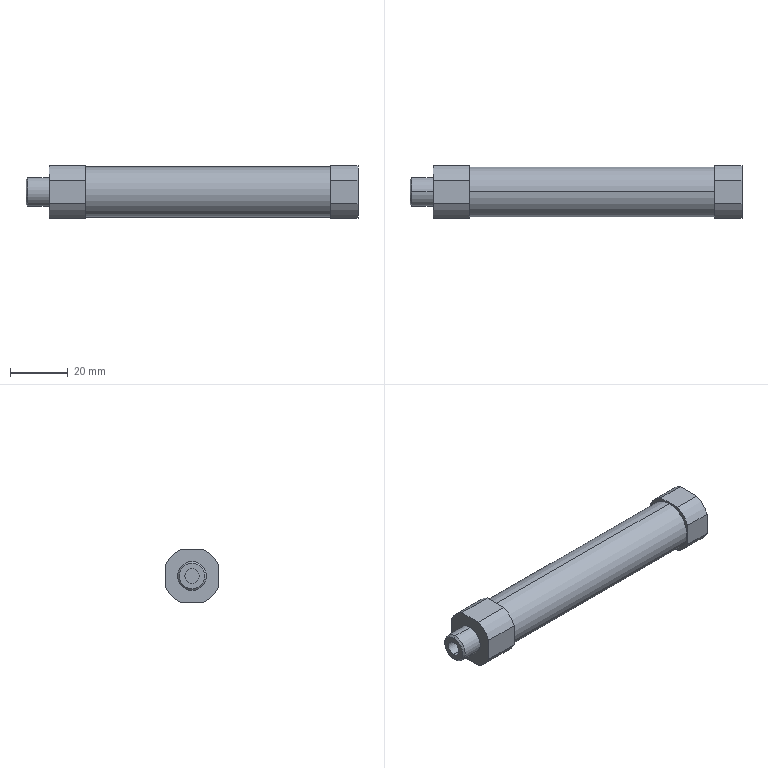Part | SolidWorks | features RefAxis 6, ICE 3, RevCut 3, 3DProfileFeature 2, Revolution 1 | 1 solid | 45 faces | box 115 x 18.3 x 18.3 mm | volume 13708 mm3 | cylinder 20 | plane 15 | cone 10 | commonest cylinder face diameters 20 x8 4.134 x4 5 x2 10 x2 16 x2 17.4 x2
STEP:
#1=CARTESIAN_POINT('',(77.5,0.,-8.));
#2=VERTEX_POINT('',#1);
#3=CARTESIAN_POINT('',(77.5,0.,8.));
#4=VERTEX_POINT('',#3);
#5=CARTESIAN_POINT('',(77.5,0.,0.));
#6=DIRECTION('',(-1.,0.,0.));
#7=DIRECTION('',(0.,0.,1.));
#8=AXIS2_PLACEMENT_3D('',#5,#6,#7);
#9=CIRCLE('',#8,8.);
#10=EDGE_CURVE('',#2,#4,#9,.T.);
#11=ORIENTED_EDGE('',*,*,#10,.F.);
#12=CARTESIAN_POINT('',(12.5,0.,-8.));
#13=VERTEX_POINT('',#12);
#14=CARTESIAN_POINT('',(50.,0.,-8.));
#15=DIRECTION('',(-1.,0.,0.));
#16=VECTOR('',#15,1000.);
#17=LINE('',#14,#16);
#18=EDGE_CURVE('',#2,#13,#17,.T.);
#19=ORIENTED_EDGE('',*,*,#18,.T.);
#20=CARTESIAN_POINT('',(12.5,0.,8.));
#21=VERTEX_POINT('',#20);
#22=CARTESIAN_POINT('',(12.5,0.,0.));
#23=DIRECTION('',(-1.,0.,0.));
#24=DIRECTION('',(0.,0.,1.));
#25=AXIS2_PLACEMENT_3D('',#22,#23,#24);
#26=CIRCLE('',#25,8.);
#27=EDGE_CURVE('',#13,#21,#26,.T.);
#28=ORIENTED_EDGE('',*,*,#27,.T.);
#29=CARTESIAN_POINT('',(50.,0.,8.));
#30=DIRECTION('',(-1.,0.,0.));
#31=VECTOR('',#30,1000.);
#32=LINE('',#29,#31);
#33=EDGE_CURVE('',#4,#21,#32,.T.);
#34=ORIENTED_EDGE('',*,*,#33,.F.);
#35=EDGE_LOOP('',(#11,#19,#28,#34));
#36=FACE_OUTER_BOUND('',#35,.T.);
#37=CARTESIAN_POINT('',(50.,0.,0.));
#38=DIRECTION('',(-1.,0.,0.));
#39=DIRECTION('',(0.,0.,1.));
#40=AXIS2_PLACEMENT_3D('',#37,#38,#39);
#41=CYLINDRICAL_SURFACE('',#40,8.);
#42=ADVANCED_FACE('',(#36),#41,.F.);
#43=CARTESIAN_POINT('',(12.5,0.,-2.5));
#44=VERTEX_POINT('',#43);
#45=CARTESIAN_POINT('',(12.5,0.,2.5));
#46=VERTEX_POINT('',#45);
#47=CARTESIAN_POINT('',(12.5,0.,0.));
#48=DIRECTION('',(-1.,0.,0.));
#49=DIRECTION('',(0.,0.,1.));
#50=AXIS2_PLACEMENT_3D('',#47,#48,#49);
#51=CIRCLE('',#50,2.5);
#52=EDGE_CURVE('',#44,#46,#51,.T.);
#53=ORIENTED_EDGE('',*,*,#52,.F.);
#54=CARTESIAN_POINT('',(-8.,0.,-2.5));
#55=VERTEX_POINT('',#54);
#56=CARTESIAN_POINT('',(50.,0.,-2.5));
#57=DIRECTION('',(-1.,0.,0.));
#58=VECTOR('',#57,1000.);
#59=LINE('',#56,#58);
#60=EDGE_CURVE('',#44,#55,#59,.T.);
#61=ORIENTED_EDGE('',*,*,#60,.T.);
#62=CARTESIAN_POINT('',(-8.,0.,2.5));
#63=VERTEX_POINT('',#62);
#64=CARTESIAN_POINT('',(-8.,0.,0.));
#65=DIRECTION('',(-1.,0.,0.));
#66=DIRECTION('',(0.,0.,1.));
#67=AXIS2_PLACEMENT_3D('',#64,#65,#66);
#68=CIRCLE('',#67,2.5);
#69=EDGE_CURVE('',#55,#63,#68,.T.);
#70=ORIENTED_EDGE('',*,*,#69,.T.);
#71=CARTESIAN_POINT('',(50.,0.,2.5));
#72=DIRECTION('',(-1.,0.,0.));
#73=VECTOR('',#72,1000.);
#74=LINE('',#71,#73);
#75=EDGE_CURVE('',#46,#63,#74,.T.);
#76=ORIENTED_EDGE('',*,*,#75,.F.);
#77=EDGE_LOOP('',(#53,#61,#70,#76));
#78=FACE_OUTER_BOUND('',#77,.T.);
#79=CARTESIAN_POINT('',(50.,0.,0.));
#80=DIRECTION('',(-1.,0.,0.));
#81=DIRECTION('',(0.,0.,1.));
#82=AXIS2_PLACEMENT_3D('',#79,#80,#81);
#83=CYLINDRICAL_SURFACE('',#82,2.5);
#84=ADVANCED_FACE('',(#78),#83,.F.);
#85=CARTESIAN_POINT('',(102.,2.457,0.));
#86=VERTEX_POINT('',#85);
#87=CARTESIAN_POINT('',(102.,3.65,2.067));
#88=VERTEX_POINT('',#87);
#89=CARTESIAN_POINT('',(102.,3.65,2.067));
#90=DIRECTION('',(0.,0.5,0.866));
#91=VECTOR('',#90,1000.);
#92=LINE('',#89,#91);
#93=EDGE_CURVE('',#86,#88,#92,.T.);
#94=ORIENTED_EDGE('',*,*,#93,.F.);
#95=CARTESIAN_POINT('',(102.,3.65,-2.067));
#96=VERTEX_POINT('',#95);
#97=CARTESIAN_POINT('',(102.,3.65,-2.067));
#98=DIRECTION('',(0.,0.5,-0.866));
#99=VECTOR('',#98,1000.);
#100=LINE('',#97,#99);
#101=EDGE_CURVE('',#86,#96,#100,.T.);
#102=ORIENTED_EDGE('',*,*,#101,.T.);
#103=CARTESIAN_POINT('',(102.,3.65,0.));
#104=DIRECTION('',(0.,-1.,0.));
#105=DIRECTION('',(0.,0.,-1.));
#106=AXIS2_PLACEMENT_3D('',#103,#104,#105);
#107=CIRCLE('',#106,2.067);
#108=EDGE_CURVE('',#88,#96,#107,.T.);
#109=ORIENTED_EDGE('',*,*,#108,.F.);
#110=EDGE_LOOP('',(#94,#102,#109));
#111=FACE_OUTER_BOUND('',#110,.T.);
#112=CARTESIAN_POINT('',(102.,3.65,0.));
#113=DIRECTION('',(0.,1.,0.));
#114=DIRECTION('',(0.,0.,1.));
#115=AXIS2_PLACEMENT_3D('',#112,#113,#114);
#116=CONICAL_SURFACE('',#115,2.067,1.047);
#117=ADVANCED_FACE('',(#111),#116,.F.);
#118=CARTESIAN_POINT('',(102.,8.717,2.067));
#119=VERTEX_POINT('',#118);
#120=CARTESIAN_POINT('',(102.,8.717,-2.067));
#121=VERTEX_POINT('',#120);
#122=CARTESIAN_POINT('',(102.,8.717,0.));
#123=DIRECTION('',(0.,-1.,0.));
#124=DIRECTION('',(0.,0.,-1.));
#125=AXIS2_PLACEMENT_3D('',#122,#123,#124);
#126=CIRCLE('',#125,2.067);
#127=EDGE_CURVE('',#119,#121,#126,.T.);
#128=ORIENTED_EDGE('',*,*,#127,.F.);
#129=CARTESIAN_POINT('',(102.,9.15,2.067));
#130=DIRECTION('',(0.,-1.,0.));
#131=VECTOR('',#130,1000.);
#132=LINE('',#129,#131);
#133=EDGE_CURVE('',#119,#88,#132,.T.);
#134=ORIENTED_EDGE('',*,*,#133,.T.);
#135=ORIENTED_EDGE('',*,*,#108,.T.);
#136=CARTESIAN_POINT('',(102.,9.15,-2.067));
#137=DIRECTION('',(0.,-1.,0.));
#138=VECTOR('',#137,1000.);
#139=LINE('',#136,#138);
#140=EDGE_CURVE('',#121,#96,#139,.T.);
#141=ORIENTED_EDGE('',*,*,#140,.F.);
#142=EDGE_LOOP('',(#128,#134,#135,#141));
#143=FACE_OUTER_BOUND('',#142,.T.);
#144=CARTESIAN_POINT('',(102.,9.15,0.));
#145=DIRECTION('',(0.,-1.,0.));
#146=DIRECTION('',(0.,0.,-1.));
#147=AXIS2_PLACEMENT_3D('',#144,#145,#146);
#148=CYLINDRICAL_SURFACE('',#147,2.067);
#149=ADVANCED_FACE('',(#143),#148,.F.);
#150=ORIENTED_EDGE('',*,*,#127,.T.);
#151=CARTESIAN_POINT('',(102.,9.15,-2.5));
#152=VERTEX_POINT('',#151);
#153=CARTESIAN_POINT('',(102.,9.15,-2.5));
#154=DIRECTION('',(0.,0.7071,-0.7071));
#155=VECTOR('',#154,1000.);
#156=LINE('',#153,#155);
#157=EDGE_CURVE('',#121,#152,#156,.T.);
#158=ORIENTED_EDGE('',*,*,#157,.T.);
#159=CARTESIAN_POINT('',(102.,9.15,2.5));
#160=VERTEX_POINT('',#159);
#161=CARTESIAN_POINT('',(102.,9.15,0.));
#162=DIRECTION('',(0.,-1.,0.));
#163=DIRECTION('',(0.,0.,-1.));
#164=AXIS2_PLACEMENT_3D('',#161,#162,#163);
#165=CIRCLE('',#164,2.5);
#166=EDGE_CURVE('',#160,#152,#165,.T.);
#167=ORIENTED_EDGE('',*,*,#166,.F.);
#168=CARTESIAN_POINT('',(102.,9.15,2.5));
#169=DIRECTION('',(0.,0.7071,0.7071));
#170=VECTOR('',#169,1000.);
#171=LINE('',#168,#170);
#172=EDGE_CURVE('',#119,#160,#171,.T.);
#173=ORIENTED_EDGE('',*,*,#172,.F.);
#174=EDGE_LOOP('',(#150,#158,#167,#173));
#175=FACE_OUTER_BOUND('',#174,.T.);
#176=CARTESIAN_POINT('',(102.,9.15,0.));
#177=DIRECTION('',(0.,1.,0.));
#178=DIRECTION('',(0.,0.,1.));
#179=AXIS2_PLACEMENT_3D('',#176,#177,#178);
#180=CONICAL_SURFACE('',#179,2.5,0.7854);
#181=ADVANCED_FACE('',(#175),#180,.F.);
#182=CARTESIAN_POINT('',(8.,8.717,2.067));
#183=VERTEX_POINT('',#182);
#184=CARTESIAN_POINT('',(8.,8.717,-2.067));
#185=VERTEX_POINT('',#184);
#186=CARTESIAN_POINT('',(8.,8.717,0.));
#187=DIRECTION('',(0.,-1.,0.));
#188=DIRECTION('',(0.,0.,-1.));
#189=AXIS2_PLACEMENT_3D('',#186,#187,#188);
#190=CIRCLE('',#189,2.067);
#191=EDGE_CURVE('',#183,#185,#190,.T.);
#192=ORIENTED_EDGE('',*,*,#191,.F.);
#193=CARTESIAN_POINT('',(8.,3.65,2.067));
#194=VERTEX_POINT('',#193);
#195=CARTESIAN_POINT('',(8.,9.15,2.067));
#196=DIRECTION('',(0.,-1.,0.));
#197=VECTOR('',#196,1000.);
#198=LINE('',#195,#197);
#199=EDGE_CURVE('',#183,#194,#198,.T.);
#200=ORIENTED_EDGE('',*,*,#199,.T.);
#201=CARTESIAN_POINT('',(8.,3.65,-2.067));
#202=VERTEX_POINT('',#201);
#203=CARTESIAN_POINT('',(8.,3.65,0.));
#204=DIRECTION('',(0.,-1.,0.));
#205=DIRECTION('',(0.,0.,-1.));
#206=AXIS2_PLACEMENT_3D('',#203,#204,#205);
#207=CIRCLE('',#206,2.067);
#208=EDGE_CURVE('',#194,#202,#207,.T.);
#209=ORIENTED_EDGE('',*,*,#208,.T.);
#210=CARTESIAN_POINT('',(8.,9.15,-2.067));
#211=DIRECTION('',(0.,-1.,0.));
#212=VECTOR('',#211,1000.);
#213=LINE('',#210,#212);
#214=EDGE_CURVE('',#185,#202,#213,.T.);
#215=ORIENTED_EDGE('',*,*,#214,.F.);
#216=EDGE_LOOP('',(#192,#200,#209,#215));
#217=FACE_OUTER_BOUND('',#216,.T.);
#218=CARTESIAN_POINT('',(8.,9.15,0.));
#219=DIRECTION('',(0.,-1.,0.));
#220=DIRECTION('',(0.,0.,-1.));
#221=AXIS2_PLACEMENT_3D('',#218,#219,#220);
#222=CYLINDRICAL_SURFACE('',#221,2.067);
#223=ADVANCED_FACE('',(#217),#222,.F.);
#224=ORIENTED_EDGE('',*,*,#191,.T.);
#225=CARTESIAN_POINT('',(8.,9.15,-2.5));
#226=VERTEX_POINT('',#225);
#227=CARTESIAN_POINT('',(8.,9.15,-2.5));
#228=DIRECTION('',(0.,0.7071,-0.7071));
#229=VECTOR('',#228,1000.);
#230=LINE('',#227,#229);
#231=EDGE_CURVE('',#185,#226,#230,.T.);
#232=ORIENTED_EDGE('',*,*,#231,.T.);
#233=CARTESIAN_POINT('',(8.,9.15,2.5));
#234=VERTEX_POINT('',#233);
#235=CARTESIAN_POINT('',(8.,9.15,0.));
#236=DIRECTION('',(0.,-1.,0.));
#237=DIRECTION('',(0.,0.,-1.));
#238=AXIS2_PLACEMENT_3D('',#235,#236,#237);
#239=CIRCLE('',#238,2.5);
#240=EDGE_CURVE('',#234,#226,#239,.T.);
#241=ORIENTED_EDGE('',*,*,#240,.F.);
#242=CARTESIAN_POINT('',(8.,9.15,2.5));
#243=DIRECTION('',(0.,0.7071,0.7071));
#244=VECTOR('',#243,1000.);
#245=LINE('',#242,#244);
#246=EDGE_CURVE('',#183,#234,#245,.T.);
#247=ORIENTED_EDGE('',*,*,#246,.F.);
#248=EDGE_LOOP('',(#224,#232,#241,#247));
#249=FACE_OUTER_BOUND('',#248,.T.);
#250=CARTESIAN_POINT('',(8.,9.15,0.));
#251=DIRECTION('',(0.,1.,0.));
#252=DIRECTION('',(0.,0.,1.));
#253=AXIS2_PLACEMENT_3D('',#250,#251,#252);
#254=CONICAL_SURFACE('',#253,2.5,0.7854);
#255=ADVANCED_FACE('',(#249),#254,.F.);
#256=CARTESIAN_POINT('',(97.5,0.,-8.7));
#257=VERTEX_POINT('',#256);
#258=CARTESIAN_POINT('',(97.5,0.,8.7));
#259=VERTEX_POINT('',#258);
#260=CARTESIAN_POINT('',(97.5,0.,0.));
#261=DIRECTION('',(1.,0.,0.));
#262=DIRECTION('',(0.,0.,-1.));
#263=AXIS2_PLACEMENT_3D('',#260,#261,#262);
#264=CIRCLE('',#263,8.7);
#265=EDGE_CURVE('',#257,#259,#264,.T.);
#266=ORIENTED_EDGE('',*,*,#265,.F.);
#267=CARTESIAN_POINT('',(12.5,0.,-8.7));
#268=VERTEX_POINT('',#267);
#269=CARTESIAN_POINT('',(97.5,0.,-8.7));
#270=DIRECTION('',(-1.,0.,0.));
#271=VECTOR('',#270,1000.);
#272=LINE('',#269,#271);
#273=EDGE_CURVE('',#257,#268,#272,.T.);
#274=ORIENTED_EDGE('',*,*,#273,.T.);
#275=CARTESIAN_POINT('',(12.5,0.,8.7));
#276=VERTEX_POINT('',#275);
#277=CARTESIAN_POINT('',(12.5,0.,0.));
#278=DIRECTION('',(1.,0.,0.));
#279=DIRECTION('',(0.,0.,-1.));
#280=AXIS2_PLACEMENT_3D('',#277,#278,#279);
#281=CIRCLE('',#280,8.7);
#282=EDGE_CURVE('',#268,#276,#281,.T.);
#283=ORIENTED_EDGE('',*,*,#282,.T.);
#284=CARTESIAN_POINT('',(97.5,0.,8.7));
#285=DIRECTION('',(-1.,0.,0.));
#286=VECTOR('',#285,1000.);
#287=LINE('',#284,#286);
#288=EDGE_CURVE('',#259,#276,#287,.T.);
#289=ORIENTED_EDGE('',*,*,#288,.F.);
#290=EDGE_LOOP('',(#266,#274,#283,#289));
#291=FACE_OUTER_BOUND('',#290,.T.);
#292=CARTESIAN_POINT('',(97.5,0.,0.));
#293=DIRECTION('',(-1.,0.,0.));
#294=DIRECTION('',(0.,0.,1.));
#295=AXIS2_PLACEMENT_3D('',#292,#293,#294);
#296=CYLINDRICAL_SURFACE('',#295,8.7);
#297=ADVANCED_FACE('',(#291),#296,.T.);
#298=CARTESIAN_POINT('',(0.,0.,-5.));
#299=VERTEX_POINT('',#298);
#300=CARTESIAN_POINT('',(0.,0.,5.));
#301=VERTEX_POINT('',#300);
#302=CARTESIAN_POINT('',(0.,0.,0.));
#303=DIRECTION('',(1.,0.,0.));
#304=DIRECTION('',(0.,0.,-1.));
#305=AXIS2_PLACEMENT_3D('',#302,#303,#304);
#306=CIRCLE('',#305,5.);
#307=EDGE_CURVE('',#299,#301,#306,.T.);
#308=ORIENTED_EDGE('',*,*,#307,.F.);
#309=CARTESIAN_POINT('',(-7.386,0.,-5.));
#310=VERTEX_POINT('',#309);
#311=CARTESIAN_POINT('',(0.,0.,-5.));
#312=DIRECTION('',(-1.,0.,0.));
#313=VECTOR('',#312,1000.);
#314=LINE('',#311,#313);
#315=EDGE_CURVE('',#299,#310,#314,.T.);
#316=ORIENTED_EDGE('',*,*,#315,.T.);
#317=CARTESIAN_POINT('',(-7.386,0.,5.));
#318=VERTEX_POINT('',#317);
#319=CARTESIAN_POINT('',(-7.386,0.,0.));
#320=DIRECTION('',(-1.,0.,0.));
#321=DIRECTION('',(0.,0.,1.));
#322=AXIS2_PLACEMENT_3D('',#319,#320,#321);
#323=CIRCLE('',#322,5.);
#324=EDGE_CURVE('',#318,#310,#323,.T.);
#325=ORIENTED_EDGE('',*,*,#324,.F.);
#326=CARTESIAN_POINT('',(0.,0.,5.));
#327=DIRECTION('',(-1.,0.,0.));
#328=VECTOR('',#327,1000.);
#329=LINE('',#326,#328);
#330=EDGE_CURVE('',#301,#318,#329,.T.);
#331=ORIENTED_EDGE('',*,*,#330,.F.);
#332=EDGE_LOOP('',(#308,#316,#325,#331));
#333=FACE_OUTER_BOUND('',#332,.T.);
#334=CARTESIAN_POINT('',(0.,0.,0.));
#335=DIRECTION('',(-1.,0.,0.));
#336=DIRECTION('',(0.,0.,1.));
#337=AXIS2_PLACEMENT_3D('',#334,#335,#336);
#338=CYLINDRICAL_SURFACE('',#337,5.);
#339=ADVANCED_FACE('',(#333),#338,.T.);
#340=CARTESIAN_POINT('',(-8.,0.,4.386));
#341=VERTEX_POINT('',#340);
#342=CARTESIAN_POINT('',(-8.,0.,-4.386));
#343=VERTEX_POINT('',#342);
#344=CARTESIAN_POINT('',(-8.,0.,0.));
#345=DIRECTION('',(-1.,0.,0.));
#346=DIRECTION('',(0.,0.,1.));
#347=AXIS2_PLACEMENT_3D('',#344,#345,#346);
#348=CIRCLE('',#347,4.386);
#349=EDGE_CURVE('',#341,#343,#348,.T.);
#350=ORIENTED_EDGE('',*,*,#349,.F.);
#351=CARTESIAN_POINT('',(-7.386,0.,5.));
#352=DIRECTION('',(0.7071,0.,0.7071));
#353=VECTOR('',#352,1000.);
#354=LINE('',#351,#353);
#355=EDGE_CURVE('',#341,#318,#354,.T.);
#356=ORIENTED_EDGE('',*,*,#355,.T.);
#357=ORIENTED_EDGE('',*,*,#324,.T.);
#358=CARTESIAN_POINT('',(-7.386,0.,-5.));
#359=DIRECTION('',(0.7071,0.,-0.7071));
#360=VECTOR('',#359,1000.);
#361=LINE('',#358,#360);
#362=EDGE_CURVE('',#343,#310,#361,.T.);
#363=ORIENTED_EDGE('',*,*,#362,.F.);
#364=EDGE_LOOP('',(#350,#356,#357,#363));
#365=FACE_OUTER_BOUND('',#364,.T.);
#366=CARTESIAN_POINT('',(-7.386,0.,0.));
#367=DIRECTION('',(1.,0.,0.));
#368=DIRECTION('',(0.,0.,-1.));
#369=AXIS2_PLACEMENT_3D('',#366,#367,#368);
#370=CONICAL_SURFACE('',#369,5.,0.7854);
#371=ADVANCED_FACE('',(#365),#370,.T.);
#372=CARTESIAN_POINT('',(8.,2.499,0.07328));
#373=VERTEX_POINT('',#372);
#374=CARTESIAN_POINT('',(8.,2.499,-0.07328));
#375=VERTEX_POINT('',#374);
#376=CARTESIAN_POINT('',(8.,2.499,0.07328));
#377=CARTESIAN_POINT('',(7.993,2.499,0.07328));
#378=CARTESIAN_POINT('',(7.987,2.499,0.07242));
#379=CARTESIAN_POINT('',(7.98,2.499,0.07073));
#380=CARTESIAN_POINT('',(7.972,2.499,0.06853));
#381=CARTESIAN_POINT('',(7.964,2.499,0.06486));
#382=CARTESIAN_POINT('',(7.957,2.499,0.06));
#383=CARTESIAN_POINT('',(7.95,2.499,0.0552));
#384=CARTESIAN_POINT('',(7.944,2.5,0.0491));
#385=CARTESIAN_POINT('',(7.939,2.5,0.0422));
#386=CARTESIAN_POINT('',(7.934,2.5,0.03545));
#387=CARTESIAN_POINT('',(7.93,2.5,0.02775));
#388=CARTESIAN_POINT('',(7.928,2.5,0.01976));
#389=CARTESIAN_POINT('',(7.925,2.5,0.01195));
#390=CARTESIAN_POINT('',(7.924,2.5,0.003644));
#391=CARTESIAN_POINT('',(7.925,2.5,-0.004461));
#392=CARTESIAN_POINT('',(7.925,2.5,-0.01245));
#393=CARTESIAN_POINT('',(7.927,2.5,-0.02046));
#394=CARTESIAN_POINT('',(7.93,2.5,-0.02784));
#395=CARTESIAN_POINT('',(7.934,2.5,-0.03523));
#396=CARTESIAN_POINT('',(7.938,2.5,-0.04219));
#397=CARTESIAN_POINT('',(7.943,2.5,-0.04817));
#398=CARTESIAN_POINT('',(7.949,2.499,-0.05426));
#399=CARTESIAN_POINT('',(7.955,2.499,-0.0595));
#400=CARTESIAN_POINT('',(7.963,2.499,-0.0635));
#401=CARTESIAN_POINT('',(7.967,2.499,-0.066));
#402=CARTESIAN_POINT('',(7.972,2.499,-0.06805));
#403=CARTESIAN_POINT('',(7.977,2.499,-0.06961));
#404=CARTESIAN_POINT('',(7.984,2.499,-0.07203));
#405=CARTESIAN_POINT('',(7.992,2.499,-0.07328));
#406=CARTESIAN_POINT('',(8.,2.499,-0.07328));
#407=B_SPLINE_CURVE_WITH_KNOTS('',3,(#376,#377,#378,#379,#380,#381,#382,#383,#384,#385,#386,#387,#388,#389,#390,#391,#392,#393,#394,#395,#396,#397,#398,#399,#400,#401,#402,#403,#404,#405,#406),.UNSPECIFIED.,.F.,.F.,(4,3,3,3,3,3,3,3,3,3,4),(0.0002557,0.0002755,0.0003013,0.0003269,0.0003518,0.0003762,0.0004002,0.0004242,0.0004487,0.0004639,0.0004876),.UNSPECIFIED.);
#408=EDGE_CURVE('',#373,#375,#407,.T.);
#409=ORIENTED_EDGE('',*,*,#408,.T.);
#410=CARTESIAN_POINT('',(8.,3.65,-2.067));
#411=DIRECTION('',(0.,0.5,-0.866));
#412=VECTOR('',#411,1000.);
#413=LINE('',#410,#412);
#414=EDGE_CURVE('',#375,#202,#413,.T.);
#415=ORIENTED_EDGE('',*,*,#414,.T.);
#416=ORIENTED_EDGE('',*,*,#208,.F.);
#417=CARTESIAN_POINT('',(8.,3.65,2.067));
#418=DIRECTION('',(0.,0.5,0.866));
#419=VECTOR('',#418,1000.);
#420=LINE('',#417,#419);
#421=EDGE_CURVE('',#373,#194,#420,.T.);
#422=ORIENTED_EDGE('',*,*,#421,.F.);
#423=EDGE_LOOP('',(#409,#415,#416,#422));
#424=FACE_OUTER_BOUND('',#423,.T.);
#425=CARTESIAN_POINT('',(8.,3.65,0.));
#426=DIRECTION('',(0.,1.,0.));
#427=DIRECTION('',(0.,0.,1.));
#428=AXIS2_PLACEMENT_3D('',#425,#426,#427);
#429=CONICAL_SURFACE('',#428,2.067,1.047);
#430=ADVANCED_FACE('',(#424),#429,.F.);
#431=CARTESIAN_POINT('',(-8.,0.,0.));
#432=DIRECTION('',(-1.,0.,0.));
#433=DIRECTION('',(0.,0.,1.));
#434=AXIS2_PLACEMENT_3D('',#431,#432,#433);
#435=CIRCLE('',#434,4.386);
#436=EDGE_CURVE('',#343,#341,#435,.T.);
#437=ORIENTED_EDGE('',*,*,#436,.T.);
#438=ORIENTED_EDGE('',*,*,#349,.T.);
#439=EDGE_LOOP('',(#437,#438));
#440=FACE_OUTER_BOUND('',#439,.T.);
#441=CARTESIAN_POINT('',(-8.,0.,0.));
#442=DIRECTION('',(-1.,0.,0.));
#443=DIRECTION('',(0.,0.,1.));
#444=AXIS2_PLACEMENT_3D('',#441,#442,#443);
#445=CIRCLE('',#444,2.5);
#446=EDGE_CURVE('',#63,#55,#445,.T.);
#447=ORIENTED_EDGE('',*,*,#446,.F.);
#448=ORIENTED_EDGE('',*,*,#69,.F.);
#449=EDGE_LOOP('',(#447,#448));
#450=FACE_BOUND('',#449,.T.);
#451=CARTESIAN_POINT('',(-8.,0.,0.));
#452=DIRECTION('',(1.,0.,0.));
#453=DIRECTION('',(0.,0.,-1.));
#454=AXIS2_PLACEMENT_3D('',#451,#452,#453);
#455=PLANE('',#454);
#456=ADVANCED_FACE('',(#440,#450),#455,.F.);
#457=ORIENTED_EDGE('',*,*,#414,.F.);
#458=CARTESIAN_POINT('',(8.,2.499,-0.07328));
#459=CARTESIAN_POINT('',(8.001,2.499,-0.07328));
#460=CARTESIAN_POINT('',(8.001,2.499,-0.07327));
#461=CARTESIAN_POINT('',(8.002,2.499,-0.07325));
#462=CARTESIAN_POINT('',(8.011,2.499,-0.07303));
#463=CARTESIAN_POINT('',(8.019,2.499,-0.07132));
#464=CARTESIAN_POINT('',(8.027,2.499,-0.06825));
#465=CARTESIAN_POINT('',(8.035,2.499,-0.06519));
#466=CARTESIAN_POINT('',(8.043,2.499,-0.06069));
#467=CARTESIAN_POINT('',(8.05,2.499,-0.05511));
#468=CARTESIAN_POINT('',(8.056,2.5,-0.04962));
#469=CARTESIAN_POINT('',(8.062,2.5,-0.04292));
#470=CARTESIAN_POINT('',(8.066,2.5,-0.03556));
#471=CARTESIAN_POINT('',(8.07,2.5,-0.02839));
#472=CARTESIAN_POINT('',(8.073,2.5,-0.0204));
#473=CARTESIAN_POINT('',(8.074,2.5,-0.01226));
#474=CARTESIAN_POINT('',(8.075,2.5,-0.004311));
#475=CARTESIAN_POINT('',(8.075,2.5,0.003993));
#476=CARTESIAN_POINT('',(8.074,2.5,0.01195));
#477=CARTESIAN_POINT('',(8.073,2.5,0.01983));
#478=CARTESIAN_POINT('',(8.07,2.5,0.02759));
#479=CARTESIAN_POINT('',(8.066,2.5,0.0346));
#480=CARTESIAN_POINT('',(8.062,2.5,0.04166));
#481=CARTESIAN_POINT('',(8.057,2.5,0.04815));
#482=CARTESIAN_POINT('',(8.051,2.499,0.05358));
#483=CARTESIAN_POINT('',(8.045,2.499,0.05912));
#484=CARTESIAN_POINT('',(8.038,2.499,0.06369));
#485=CARTESIAN_POINT('',(8.031,2.499,0.06696));
#486=CARTESIAN_POINT('',(8.023,2.499,0.07032));
#487=CARTESIAN_POINT('',(8.014,2.499,0.07239));
#488=CARTESIAN_POINT('',(8.006,2.499,0.07305));
#489=CARTESIAN_POINT('',(8.004,2.499,0.0732));
#490=CARTESIAN_POINT('',(8.002,2.499,0.07328));
#491=CARTESIAN_POINT('',(8.,2.499,0.07328));
#492=B_SPLINE_CURVE_WITH_KNOTS('',3,(#458,#459,#460,#461,#462,#463,#464,#465,#466,#467,#468,#469,#470,#471,#472,#473,#474,#475,#476,#477,#478,#479,#480,#481,#482,#483,#484,#485,#486,#487,#488,#489,#490,#491),.UNSPECIFIED.,.F.,.F.,(4,3,3,3,3,3,3,3,3,3,3,4),(0.00002375,0.00002578,0.00005157,0.00007735,0.0001027,0.0001275,0.0001517,0.0001757,0.0001998,0.0002245,0.0002498,0.0002557),.UNSPECIFIED.);
#493=EDGE_CURVE('',#375,#373,#492,.T.);
#494=ORIENTED_EDGE('',*,*,#493,.T.);
#495=ORIENTED_EDGE('',*,*,#421,.T.);
#496=CARTESIAN_POINT('',(8.,3.65,0.));
#497=DIRECTION('',(0.,-1.,0.));
#498=DIRECTION('',(0.,0.,-1.));
#499=AXIS2_PLACEMENT_3D('',#496,#497,#498);
#500=CIRCLE('',#499,2.067);
#501=EDGE_CURVE('',#202,#194,#500,.T.);
#502=ORIENTED_EDGE('',*,*,#501,.F.);
#503=EDGE_LOOP('',(#457,#494,#495,#502));
#504=FACE_OUTER_BOUND('',#503,.T.);
#505=CARTESIAN_POINT('',(8.,3.65,0.));
#506=DIRECTION('',(0.,1.,0.));
#507=DIRECTION('',(0.,0.,1.));
#508=AXIS2_PLACEMENT_3D('',#505,#506,#507);
#509=CONICAL_SURFACE('',#508,2.067,1.047);
#510=ADVANCED_FACE('',(#504),#509,.F.);
#511=CARTESIAN_POINT('',(97.5,9.15,-4.035));
#512=VERTEX_POINT('',#511);
#513=CARTESIAN_POINT('',(97.5,9.15,4.035));
#514=VERTEX_POINT('',#513);
#515=CARTESIAN_POINT('',(97.5,9.15,-4.035));
#516=DIRECTION('',(0.,0.,1.));
#517=VECTOR('',#516,1000.);
#518=LINE('',#515,#517);
#519=EDGE_CURVE('',#512,#514,#518,.T.);
#520=ORIENTED_EDGE('',*,*,#519,.T.);
#521=CARTESIAN_POINT('',(107.,9.15,4.035));
#522=VERTEX_POINT('',#521);
#523=CARTESIAN_POINT('',(107.,9.15,4.035));
#524=DIRECTION('',(-1.,0.,0.));
#525=VECTOR('',#524,1000.);
#526=LINE('',#523,#525);
#527=EDGE_CURVE('',#522,#514,#526,.T.);
#528=ORIENTED_EDGE('',*,*,#527,.F.);
#529=CARTESIAN_POINT('',(107.,9.15,-4.035));
#530=VERTEX_POINT('',#529);
#531=CARTESIAN_POINT('',(107.,9.15,-4.035));
#532=DIRECTION('',(0.,0.,1.));
#533=VECTOR('',#532,1000.);
#534=LINE('',#531,#533);
#535=EDGE_CURVE('',#530,#522,#534,.T.);
#536=ORIENTED_EDGE('',*,*,#535,.F.);
#537=CARTESIAN_POINT('',(107.,9.15,-4.035));
#538=DIRECTION('',(-1.,0.,0.));
#539=VECTOR('',#538,1000.);
#540=LINE('',#537,#539);
#541=EDGE_CURVE('',#530,#512,#540,.T.);
#542=ORIENTED_EDGE('',*,*,#541,.T.);
#543=EDGE_LOOP('',(#520,#528,#536,#542));
#544=FACE_OUTER_BOUND('',#543,.T.);
#545=ORIENTED_EDGE('',*,*,#166,.T.);
#546=CARTESIAN_POINT('',(102.,9.15,0.));
#547=DIRECTION('',(0.,-1.,0.));
#548=DIRECTION('',(0.,0.,-1.));
#549=AXIS2_PLACEMENT_3D('',#546,#547,#548);
#550=CIRCLE('',#549,2.5);
#551=EDGE_CURVE('',#152,#160,#550,.T.);
#552=ORIENTED_EDGE('',*,*,#551,.T.);
#553=EDGE_LOOP('',(#545,#552));
#554=FACE_BOUND('',#553,.T.);
#555=CARTESIAN_POINT('',(107.,9.15,-4.035));
#556=DIRECTION('',(0.,-1.,0.));
#557=DIRECTION('',(0.,0.,-1.));
#558=AXIS2_PLACEMENT_3D('',#555,#556,#557);
#559=PLANE('',#558);
#560=ADVANCED_FACE('',(#544,#554),#559,.F.);
#561=CARTESIAN_POINT('',(0.,9.15,-4.035));
#562=VERTEX_POINT('',#561);
#563=CARTESIAN_POINT('',(0.,9.15,4.035));
#564=VERTEX_POINT('',#563);
#565=CARTESIAN_POINT('',(0.,9.15,-4.035));
#566=DIRECTION('',(0.,0.,1.));
#567=VECTOR('',#566,1000.);
#568=LINE('',#565,#567);
#569=EDGE_CURVE('',#562,#564,#568,.T.);
#570=ORIENTED_EDGE('',*,*,#569,.T.);
#571=CARTESIAN_POINT('',(12.5,9.15,4.035));
#572=VERTEX_POINT('',#571);
#573=CARTESIAN_POINT('',(12.5,9.15,4.035));
#574=DIRECTION('',(-1.,0.,0.));
#575=VECTOR('',#574,1000.);
#576=LINE('',#573,#575);
#577=EDGE_CURVE('',#572,#564,#576,.T.);
#578=ORIENTED_EDGE('',*,*,#577,.F.);
#579=CARTESIAN_POINT('',(12.5,9.15,-4.035));
#580=VERTEX_POINT('',#579);
#581=CARTESIAN_POINT('',(12.5,9.15,-4.035));
#582=DIRECTION('',(0.,0.,1.));
#583=VECTOR('',#582,1000.);
#584=LINE('',#581,#583);
#585=EDGE_CURVE('',#580,#572,#584,.T.);
#586=ORIENTED_EDGE('',*,*,#585,.F.);
#587=CARTESIAN_POINT('',(12.5,9.15,-4.035));
#588=DIRECTION('',(-1.,0.,0.));
#589=VECTOR('',#588,1000.);
#590=LINE('',#587,#589);
#591=EDGE_CURVE('',#580,#562,#590,.T.);
#592=ORIENTED_EDGE('',*,*,#591,.T.);
#593=EDGE_LOOP('',(#570,#578,#586,#592));
#594=FACE_OUTER_BOUND('',#593,.T.);
#595=ORIENTED_EDGE('',*,*,#240,.T.);
#596=CARTESIAN_POINT('',(8.,9.15,0.));
#597=DIRECTION('',(0.,-1.,0.));
#598=DIRECTION('',(0.,0.,-1.));
#599=AXIS2_PLACEMENT_3D('',#596,#597,#598);
#600=CIRCLE('',#599,2.5);
#601=EDGE_CURVE('',#226,#234,#600,.T.);
#602=ORIENTED_EDGE('',*,*,#601,.T.);
#603=EDGE_LOOP('',(#595,#602));
#604=FACE_BOUND('',#603,.T.);
#605=CARTESIAN_POINT('',(12.5,9.15,-4.035));
#606=DIRECTION('',(0.,-1.,0.));
#607=DIRECTION('',(0.,0.,-1.));
#608=AXIS2_PLACEMENT_3D('',#605,#606,#607);
#609=PLANE('',#608);
#610=ADVANCED_FACE('',(#594,#604),#609,.F.);
#611=CARTESIAN_POINT('',(12.5,-4.035,9.15));
#612=VERTEX_POINT('',#611);
#613=CARTESIAN_POINT('',(12.5,-9.15,4.035));
#614=VERTEX_POINT('',#613);
#615=CARTESIAN_POINT('',(12.5,0.,0.));
#616=DIRECTION('',(1.,0.,0.));
#617=DIRECTION('',(0.,0.,-1.));
#618=AXIS2_PLACEMENT_3D('',#615,#616,#617);
#619=CIRCLE('',#618,10.);
#620=EDGE_CURVE('',#612,#614,#619,.T.);
#621=ORIENTED_EDGE('',*,*,#620,.T.);
#622=CARTESIAN_POINT('',(12.5,-9.15,-4.035));
#623=VERTEX_POINT('',#622);
#624=CARTESIAN_POINT('',(12.5,-9.15,4.035));
#625=DIRECTION('',(0.,0.,-1.));
#626=VECTOR('',#625,1000.);
#627=LINE('',#624,#626);
#628=EDGE_CURVE('',#614,#623,#627,.T.);
#629=ORIENTED_EDGE('',*,*,#628,.T.);
#630=CARTESIAN_POINT('',(12.5,-4.035,-9.15));
#631=VERTEX_POINT('',#630);
#632=CARTESIAN_POINT('',(12.5,0.,0.));
#633=DIRECTION('',(1.,0.,0.));
#634=DIRECTION('',(0.,0.,-1.));
#635=AXIS2_PLACEMENT_3D('',#632,#633,#634);
#636=CIRCLE('',#635,10.);
#637=EDGE_CURVE('',#623,#631,#636,.T.);
#638=ORIENTED_EDGE('',*,*,#637,.T.);
#639=CARTESIAN_POINT('',(12.5,4.035,-9.15));
#640=VERTEX_POINT('',#639);
#641=CARTESIAN_POINT('',(12.5,-4.035,-9.15));
#642=DIRECTION('',(0.,1.,0.));
#643=VECTOR('',#642,1000.);
#644=LINE('',#641,#643);
#645=EDGE_CURVE('',#631,#640,#644,.T.);
#646=ORIENTED_EDGE('',*,*,#645,.T.);
#647=CARTESIAN_POINT('',(12.5,0.,0.));
#648=DIRECTION('',(1.,0.,0.));
#649=DIRECTION('',(0.,0.,-1.));
#650=AXIS2_PLACEMENT_3D('',#647,#648,#649);
#651=CIRCLE('',#650,10.);
#652=EDGE_CURVE('',#640,#580,#651,.T.);
#653=ORIENTED_EDGE('',*,*,#652,.T.);
#654=ORIENTED_EDGE('',*,*,#585,.T.);
#655=CARTESIAN_POINT('',(12.5,4.035,9.15));
#656=VERTEX_POINT('',#655);
#657=CARTESIAN_POINT('',(12.5,0.,0.));
#658=DIRECTION('',(1.,0.,0.));
#659=DIRECTION('',(0.,0.,-1.));
#660=AXIS2_PLACEMENT_3D('',#657,#658,#659);
#661=CIRCLE('',#660,10.);
#662=EDGE_CURVE('',#572,#656,#661,.T.);
#663=ORIENTED_EDGE('',*,*,#662,.T.);
#664=CARTESIAN_POINT('',(12.5,4.035,9.15));
#665=DIRECTION('',(0.,-1.,0.));
#666=VECTOR('',#665,1000.);
#667=LINE('',#664,#666);
#668=EDGE_CURVE('',#656,#612,#667,.T.);
#669=ORIENTED_EDGE('',*,*,#668,.T.);
#670=EDGE_LOOP('',(#621,#629,#638,#646,#653,#654,#663,#669));
#671=FACE_OUTER_BOUND('',#670,.T.);
#672=CARTESIAN_POINT('',(12.5,0.,0.));
#673=DIRECTION('',(1.,0.,0.));
#674=DIRECTION('',(0.,0.,-1.));
#675=AXIS2_PLACEMENT_3D('',#672,#673,#674);
#676=CIRCLE('',#675,8.7);
#677=EDGE_CURVE('',#276,#268,#676,.T.);
#678=ORIENTED_EDGE('',*,*,#677,.F.);
#679=ORIENTED_EDGE('',*,*,#282,.F.);
#680=EDGE_LOOP('',(#678,#679));
#681=FACE_BOUND('',#680,.T.);
#682=CARTESIAN_POINT('',(12.5,0.,0.));
#683=DIRECTION('',(1.,0.,0.));
#684=DIRECTION('',(0.,0.,-1.));
#685=AXIS2_PLACEMENT_3D('',#682,#683,#684);
#686=PLANE('',#685);
#687=ADVANCED_FACE('',(#671,#681),#686,.T.);
#688=ORIENTED_EDGE('',*,*,#355,.F.);
#689=ORIENTED_EDGE('',*,*,#436,.F.);
#690=ORIENTED_EDGE('',*,*,#362,.T.);
#691=CARTESIAN_POINT('',(-7.386,0.,0.));
#692=DIRECTION('',(-1.,0.,0.));
#693=DIRECTION('',(0.,0.,1.));
#694=AXIS2_PLACEMENT_3D('',#691,#692,#693);
#695=CIRCLE('',#694,5.);
#696=EDGE_CURVE('',#310,#318,#695,.T.);
#697=ORIENTED_EDGE('',*,*,#696,.T.);
#698=EDGE_LOOP('',(#688,#689,#690,#697));
#699=FACE_OUTER_BOUND('',#698,.T.);
#700=CARTESIAN_POINT('',(-7.386,0.,0.));
#701=DIRECTION('',(1.,0.,0.));
#702=DIRECTION('',(0.,0.,-1.));
#703=AXIS2_PLACEMENT_3D('',#700,#701,#702);
#704=CONICAL_SURFACE('',#703,5.,0.7854);
#705=ADVANCED_FACE('',(#699),#704,.T.);
#706=ORIENTED_EDGE('',*,*,#315,.F.);
#707=CARTESIAN_POINT('',(0.,0.,0.));
#708=DIRECTION('',(1.,0.,0.));
#709=DIRECTION('',(0.,0.,-1.));
#710=AXIS2_PLACEMENT_3D('',#707,#708,#709);
#711=CIRCLE('',#710,5.);
#712=EDGE_CURVE('',#301,#299,#711,.T.);
#713=ORIENTED_EDGE('',*,*,#712,.F.);
#714=ORIENTED_EDGE('',*,*,#330,.T.);
#715=ORIENTED_EDGE('',*,*,#696,.F.);
#716=EDGE_LOOP('',(#706,#713,#714,#715));
#717=FACE_OUTER_BOUND('',#716,.T.);
#718=CARTESIAN_POINT('',(0.,0.,0.));
#719=DIRECTION('',(-1.,0.,0.));
#720=DIRECTION('',(0.,0.,1.));
#721=AXIS2_PLACEMENT_3D('',#718,#719,#720);
#722=CYLINDRICAL_SURFACE('',#721,5.);
#723=ADVANCED_FACE('',(#717),#722,.T.);
#724=CARTESIAN_POINT('',(0.,-4.035,9.15));
#725=VERTEX_POINT('',#724);
#726=CARTESIAN_POINT('',(0.,-9.15,4.035));
#727=VERTEX_POINT('',#726);
#728=CARTESIAN_POINT('',(0.,0.,0.));
#729=DIRECTION('',(1.,0.,0.));
#730=DIRECTION('',(0.,0.,-1.));
#731=AXIS2_PLACEMENT_3D('',#728,#729,#730);
#732=CIRCLE('',#731,10.);
#733=EDGE_CURVE('',#725,#727,#732,.T.);
#734=ORIENTED_EDGE('',*,*,#733,.F.);
#735=CARTESIAN_POINT('',(0.,4.035,9.15));
#736=VERTEX_POINT('',#735);
#737=CARTESIAN_POINT('',(0.,4.035,9.15));
#738=DIRECTION('',(0.,-1.,0.));
#739=VECTOR('',#738,1000.);
#740=LINE('',#737,#739);
#741=EDGE_CURVE('',#736,#725,#740,.T.);
#742=ORIENTED_EDGE('',*,*,#741,.F.);
#743=CARTESIAN_POINT('',(0.,0.,0.));
#744=DIRECTION('',(1.,0.,0.));
#745=DIRECTION('',(0.,0.,-1.));
#746=AXIS2_PLACEMENT_3D('',#743,#744,#745);
#747=CIRCLE('',#746,10.);
#748=EDGE_CURVE('',#564,#736,#747,.T.);
#749=ORIENTED_EDGE('',*,*,#748,.F.);
#750=ORIENTED_EDGE('',*,*,#569,.F.);
#751=CARTESIAN_POINT('',(0.,4.035,-9.15));
#752=VERTEX_POINT('',#751);
#753=CARTESIAN_POINT('',(0.,0.,0.));
#754=DIRECTION('',(1.,0.,0.));
#755=DIRECTION('',(0.,0.,-1.));
#756=AXIS2_PLACEMENT_3D('',#753,#754,#755);
#757=CIRCLE('',#756,10.);
#758=EDGE_CURVE('',#752,#562,#757,.T.);
#759=ORIENTED_EDGE('',*,*,#758,.F.);
#760=CARTESIAN_POINT('',(0.,-4.035,-9.15));
#761=VERTEX_POINT('',#760);
#762=CARTESIAN_POINT('',(0.,-4.035,-9.15));
#763=DIRECTION('',(0.,1.,0.));
#764=VECTOR('',#763,1000.);
#765=LINE('',#762,#764);
#766=EDGE_CURVE('',#761,#752,#765,.T.);
#767=ORIENTED_EDGE('',*,*,#766,.F.);
#768=CARTESIAN_POINT('',(0.,-9.15,-4.035));
#769=VERTEX_POINT('',#768);
#770=CARTESIAN_POINT('',(0.,0.,0.));
#771=DIRECTION('',(1.,0.,0.));
#772=DIRECTION('',(0.,0.,-1.));
#773=AXIS2_PLACEMENT_3D('',#770,#771,#772);
#774=CIRCLE('',#773,10.);
#775=EDGE_CURVE('',#769,#761,#774,.T.);
#776=ORIENTED_EDGE('',*,*,#775,.F.);
#777=CARTESIAN_POINT('',(0.,-9.15,4.035));
#778=DIRECTION('',(0.,0.,-1.));
#779=VECTOR('',#778,1000.);
#780=LINE('',#777,#779);
#781=EDGE_CURVE('',#727,#769,#780,.T.);
#782=ORIENTED_EDGE('',*,*,#781,.F.);
#783=EDGE_LOOP('',(#734,#742,#749,#750,#759,#767,#776,#782));
#784=FACE_OUTER_BOUND('',#783,.T.);
#785=ORIENTED_EDGE('',*,*,#712,.T.);
#786=ORIENTED_EDGE('',*,*,#307,.T.);
#787=EDGE_LOOP('',(#785,#786));
#788=FACE_BOUND('',#787,.T.);
#789=CARTESIAN_POINT('',(0.,0.,0.));
#790=DIRECTION('',(1.,0.,0.));
#791=DIRECTION('',(0.,0.,-1.));
#792=AXIS2_PLACEMENT_3D('',#789,#790,#791);
#793=PLANE('',#792);
#794=ADVANCED_FACE('',(#784,#788),#793,.F.);
#795=ORIENTED_EDGE('',*,*,#733,.T.);
#796=CARTESIAN_POINT('',(12.5,-9.15,4.035));
#797=DIRECTION('',(-1.,0.,0.));
#798=VECTOR('',#797,1000.);
#799=LINE('',#796,#798);
#800=EDGE_CURVE('',#614,#727,#799,.T.);
#801=ORIENTED_EDGE('',*,*,#800,.F.);
#802=ORIENTED_EDGE('',*,*,#620,.F.);
#803=CARTESIAN_POINT('',(12.5,-4.035,9.15));
#804=DIRECTION('',(-1.,0.,0.));
#805=VECTOR('',#804,1000.);
#806=LINE('',#803,#805);
#807=EDGE_CURVE('',#612,#725,#806,.T.);
#808=ORIENTED_EDGE('',*,*,#807,.T.);
#809=EDGE_LOOP('',(#795,#801,#802,#808));
#810=FACE_OUTER_BOUND('',#809,.T.);
#811=CARTESIAN_POINT('',(12.5,0.,0.));
#812=DIRECTION('',(-1.,0.,0.));
#813=DIRECTION('',(0.,0.,1.));
#814=AXIS2_PLACEMENT_3D('',#811,#812,#813);
#815=CYLINDRICAL_SURFACE('',#814,10.);
#816=ADVANCED_FACE('',(#810),#815,.T.);
#817=ORIENTED_EDGE('',*,*,#781,.T.);
#818=CARTESIAN_POINT('',(12.5,-9.15,-4.035));
#819=DIRECTION('',(-1.,0.,0.));
#820=VECTOR('',#819,1000.);
#821=LINE('',#818,#820);
#822=EDGE_CURVE('',#623,#769,#821,.T.);
#823=ORIENTED_EDGE('',*,*,#822,.F.);
#824=ORIENTED_EDGE('',*,*,#628,.F.);
#825=ORIENTED_EDGE('',*,*,#800,.T.);
#826=EDGE_LOOP('',(#817,#823,#824,#825));
#827=FACE_OUTER_BOUND('',#826,.T.);
#828=CARTESIAN_POINT('',(12.5,-9.15,4.035));
#829=DIRECTION('',(0.,1.,0.));
#830=DIRECTION('',(0.,0.,1.));
#831=AXIS2_PLACEMENT_3D('',#828,#829,#830);
#832=PLANE('',#831);
#833=ADVANCED_FACE('',(#827),#832,.F.);
#834=ORIENTED_EDGE('',*,*,#775,.T.);
#835=CARTESIAN_POINT('',(12.5,-4.035,-9.15));
#836=DIRECTION('',(-1.,0.,0.));
#837=VECTOR('',#836,1000.);
#838=LINE('',#835,#837);
#839=EDGE_CURVE('',#631,#761,#838,.T.);
#840=ORIENTED_EDGE('',*,*,#839,.F.);
#841=ORIENTED_EDGE('',*,*,#637,.F.);
#842=ORIENTED_EDGE('',*,*,#822,.T.);
#843=EDGE_LOOP('',(#834,#840,#841,#842));
#844=FACE_OUTER_BOUND('',#843,.T.);
#845=CARTESIAN_POINT('',(12.5,0.,0.));
#846=DIRECTION('',(-1.,0.,0.));
#847=DIRECTION('',(0.,0.,1.));
#848=AXIS2_PLACEMENT_3D('',#845,#846,#847);
#849=CYLINDRICAL_SURFACE('',#848,10.);
#850=ADVANCED_FACE('',(#844),#849,.T.);
#851=ORIENTED_EDGE('',*,*,#766,.T.);
#852=CARTESIAN_POINT('',(12.5,4.035,-9.15));
#853=DIRECTION('',(-1.,0.,0.));
#854=VECTOR('',#853,1000.);
#855=LINE('',#852,#854);
#856=EDGE_CURVE('',#640,#752,#855,.T.);
#857=ORIENTED_EDGE('',*,*,#856,.F.);
#858=ORIENTED_EDGE('',*,*,#645,.F.);
#859=ORIENTED_EDGE('',*,*,#839,.T.);
#860=EDGE_LOOP('',(#851,#857,#858,#859));
#861=FACE_OUTER_BOUND('',#860,.T.);
#862=CARTESIAN_POINT('',(12.5,-4.035,-9.15));
#863=DIRECTION('',(0.,0.,1.));
#864=DIRECTION('',(1.,0.,0.));
#865=AXIS2_PLACEMENT_3D('',#862,#863,#864);
#866=PLANE('',#865);
#867=ADVANCED_FACE('',(#861),#866,.F.);
#868=ORIENTED_EDGE('',*,*,#758,.T.);
#869=ORIENTED_EDGE('',*,*,#591,.F.);
#870=ORIENTED_EDGE('',*,*,#652,.F.);
#871=ORIENTED_EDGE('',*,*,#856,.T.);
#872=EDGE_LOOP('',(#868,#869,#870,#871));
#873=FACE_OUTER_BOUND('',#872,.T.);
#874=CARTESIAN_POINT('',(12.5,0.,0.));
#875=DIRECTION('',(-1.,0.,0.));
#876=DIRECTION('',(0.,0.,1.));
#877=AXIS2_PLACEMENT_3D('',#874,#875,#876);
#878=CYLINDRICAL_SURFACE('',#877,10.);
#879=ADVANCED_FACE('',(#873),#878,.T.);
#880=ORIENTED_EDGE('',*,*,#748,.T.);
#881=CARTESIAN_POINT('',(12.5,4.035,9.15));
#882=DIRECTION('',(-1.,0.,0.));
#883=VECTOR('',#882,1000.);
#884=LINE('',#881,#883);
#885=EDGE_CURVE('',#656,#736,#884,.T.);
#886=ORIENTED_EDGE('',*,*,#885,.F.);
#887=ORIENTED_EDGE('',*,*,#662,.F.);
#888=ORIENTED_EDGE('',*,*,#577,.T.);
#889=EDGE_LOOP('',(#880,#886,#887,#888));
#890=FACE_OUTER_BOUND('',#889,.T.);
#891=CARTESIAN_POINT('',(12.5,0.,0.));
#892=DIRECTION('',(-1.,0.,0.));
#893=DIRECTION('',(0.,0.,1.));
#894=AXIS2_PLACEMENT_3D('',#891,#892,#893);
#895=CYLINDRICAL_SURFACE('',#894,10.);
#896=ADVANCED_FACE('',(#890),#895,.T.);
#897=ORIENTED_EDGE('',*,*,#741,.T.);
#898=ORIENTED_EDGE('',*,*,#807,.F.);
#899=ORIENTED_EDGE('',*,*,#668,.F.);
#900=ORIENTED_EDGE('',*,*,#885,.T.);
#901=EDGE_LOOP('',(#897,#898,#899,#900));
#902=FACE_OUTER_BOUND('',#901,.T.);
#903=CARTESIAN_POINT('',(12.5,4.035,9.15));
#904=DIRECTION('',(0.,0.,-1.));
#905=DIRECTION('',(-1.,0.,0.));
#906=AXIS2_PLACEMENT_3D('',#903,#904,#905);
#907=PLANE('',#906);
#908=ADVANCED_FACE('',(#902),#907,.F.);
#909=ORIENTED_EDGE('',*,*,#273,.F.);
#910=CARTESIAN_POINT('',(97.5,0.,0.));
#911=DIRECTION('',(1.,0.,0.));
#912=DIRECTION('',(0.,0.,-1.));
#913=AXIS2_PLACEMENT_3D('',#910,#911,#912);
#914=CIRCLE('',#913,8.7);
#915=EDGE_CURVE('',#259,#257,#914,.T.);
#916=ORIENTED_EDGE('',*,*,#915,.F.);
#917=ORIENTED_EDGE('',*,*,#288,.T.);
#918=ORIENTED_EDGE('',*,*,#677,.T.);
#919=EDGE_LOOP('',(#909,#916,#917,#918));
#920=FACE_OUTER_BOUND('',#919,.T.);
#921=CARTESIAN_POINT('',(97.5,0.,0.));
#922=DIRECTION('',(-1.,0.,0.));
#923=DIRECTION('',(0.,0.,1.));
#924=AXIS2_PLACEMENT_3D('',#921,#922,#923);
#925=CYLINDRICAL_SURFACE('',#924,8.7);
#926=ADVANCED_FACE('',(#920),#925,.T.);
#927=CARTESIAN_POINT('',(97.5,-4.035,9.15));
#928=VERTEX_POINT('',#927);
#929=CARTESIAN_POINT('',(97.5,-9.15,4.035));
#930=VERTEX_POINT('',#929);
#931=CARTESIAN_POINT('',(97.5,0.,0.));
#932=DIRECTION('',(1.,0.,0.));
#933=DIRECTION('',(0.,0.,-1.));
#934=AXIS2_PLACEMENT_3D('',#931,#932,#933);
#935=CIRCLE('',#934,10.);
#936=EDGE_CURVE('',#928,#930,#935,.T.);
#937=ORIENTED_EDGE('',*,*,#936,.F.);
#938=CARTESIAN_POINT('',(97.5,4.035,9.15));
#939=VERTEX_POINT('',#938);
#940=CARTESIAN_POINT('',(97.5,4.035,9.15));
#941=DIRECTION('',(0.,-1.,0.));
#942=VECTOR('',#941,1000.);
#943=LINE('',#940,#942);
#944=EDGE_CURVE('',#939,#928,#943,.T.);
#945=ORIENTED_EDGE('',*,*,#944,.F.);
#946=CARTESIAN_POINT('',(97.5,0.,0.));
#947=DIRECTION('',(1.,0.,0.));
#948=DIRECTION('',(0.,0.,-1.));
#949=AXIS2_PLACEMENT_3D('',#946,#947,#948);
#950=CIRCLE('',#949,10.);
#951=EDGE_CURVE('',#514,#939,#950,.T.);
#952=ORIENTED_EDGE('',*,*,#951,.F.);
#953=ORIENTED_EDGE('',*,*,#519,.F.);
#954=CARTESIAN_POINT('',(97.5,4.035,-9.15));
#955=VERTEX_POINT('',#954);
#956=CARTESIAN_POINT('',(97.5,0.,0.));
#957=DIRECTION('',(1.,0.,0.));
#958=DIRECTION('',(0.,0.,-1.));
#959=AXIS2_PLACEMENT_3D('',#956,#957,#958);
#960=CIRCLE('',#959,10.);
#961=EDGE_CURVE('',#955,#512,#960,.T.);
#962=ORIENTED_EDGE('',*,*,#961,.F.);
#963=CARTESIAN_POINT('',(97.5,-4.035,-9.15));
#964=VERTEX_POINT('',#963);
#965=CARTESIAN_POINT('',(97.5,-4.035,-9.15));
#966=DIRECTION('',(0.,1.,0.));
#967=VECTOR('',#966,1000.);
#968=LINE('',#965,#967);
#969=EDGE_CURVE('',#964,#955,#968,.T.);
#970=ORIENTED_EDGE('',*,*,#969,.F.);
#971=CARTESIAN_POINT('',(97.5,-9.15,-4.035));
#972=VERTEX_POINT('',#971);
#973=CARTESIAN_POINT('',(97.5,0.,0.));
#974=DIRECTION('',(1.,0.,0.));
#975=DIRECTION('',(0.,0.,-1.));
#976=AXIS2_PLACEMENT_3D('',#973,#974,#975);
#977=CIRCLE('',#976,10.);
#978=EDGE_CURVE('',#972,#964,#977,.T.);
#979=ORIENTED_EDGE('',*,*,#978,.F.);
#980=CARTESIAN_POINT('',(97.5,-9.15,4.035));
#981=DIRECTION('',(0.,0.,-1.));
#982=VECTOR('',#981,1000.);
#983=LINE('',#980,#982);
#984=EDGE_CURVE('',#930,#972,#983,.T.);
#985=ORIENTED_EDGE('',*,*,#984,.F.);
#986=EDGE_LOOP('',(#937,#945,#952,#953,#962,#970,#979,#985));
#987=FACE_OUTER_BOUND('',#986,.T.);
#988=ORIENTED_EDGE('',*,*,#915,.T.);
#989=ORIENTED_EDGE('',*,*,#265,.T.);
#990=EDGE_LOOP('',(#988,#989));
#991=FACE_BOUND('',#990,.T.);
#992=CARTESIAN_POINT('',(97.5,0.,0.));
#993=DIRECTION('',(1.,0.,0.));
#994=DIRECTION('',(0.,0.,-1.));
#995=AXIS2_PLACEMENT_3D('',#992,#993,#994);
#996=PLANE('',#995);
#997=ADVANCED_FACE('',(#987,#991),#996,.F.);
#998=ORIENTED_EDGE('',*,*,#936,.T.);
#999=CARTESIAN_POINT('',(107.,-9.15,4.035));
#1000=VERTEX_POINT('',#999);
#1001=CARTESIAN_POINT('',(107.,-9.15,4.035));
#1002=DIRECTION('',(-1.,0.,0.));
#1003=VECTOR('',#1002,1000.);
#1004=LINE('',#1001,#1003);
#1005=EDGE_CURVE('',#1000,#930,#1004,.T.);
#1006=ORIENTED_EDGE('',*,*,#1005,.F.);
#1007=CARTESIAN_POINT('',(107.,-4.035,9.15));
#1008=VERTEX_POINT('',#1007);
#1009=CARTESIAN_POINT('',(107.,0.,0.));
#1010=DIRECTION('',(1.,0.,0.));
#1011=DIRECTION('',(0.,0.,-1.));
#1012=AXIS2_PLACEMENT_3D('',#1009,#1010,#1011);
#1013=CIRCLE('',#1012,10.);
#1014=EDGE_CURVE('',#1008,#1000,#1013,.T.);
#1015=ORIENTED_EDGE('',*,*,#1014,.F.);
#1016=CARTESIAN_POINT('',(107.,-4.035,9.15));
#1017=DIRECTION('',(-1.,0.,0.));
#1018=VECTOR('',#1017,1000.);
#1019=LINE('',#1016,#1018);
#1020=EDGE_CURVE('',#1008,#928,#1019,.T.);
#1021=ORIENTED_EDGE('',*,*,#1020,.T.);
#1022=EDGE_LOOP('',(#998,#1006,#1015,#1021));
#1023=FACE_OUTER_BOUND('',#1022,.T.);
#1024=CARTESIAN_POINT('',(107.,0.,0.));
#1025=DIRECTION('',(-1.,0.,0.));
#1026=DIRECTION('',(0.,0.,1.));
#1027=AXIS2_PLACEMENT_3D('',#1024,#1025,#1026);
#1028=CYLINDRICAL_SURFACE('',#1027,10.);
#1029=ADVANCED_FACE('',(#1023),#1028,.T.);
#1030=ORIENTED_EDGE('',*,*,#984,.T.);
#1031=CARTESIAN_POINT('',(107.,-9.15,-4.035));
#1032=VERTEX_POINT('',#1031);
#1033=CARTESIAN_POINT('',(107.,-9.15,-4.035));
#1034=DIRECTION('',(-1.,0.,0.));
#1035=VECTOR('',#1034,1000.);
#1036=LINE('',#1033,#1035);
#1037=EDGE_CURVE('',#1032,#972,#1036,.T.);
#1038=ORIENTED_EDGE('',*,*,#1037,.F.);
#1039=CARTESIAN_POINT('',(107.,-9.15,4.035));
#1040=DIRECTION('',(0.,0.,-1.));
#1041=VECTOR('',#1040,1000.);
#1042=LINE('',#1039,#1041);
#1043=EDGE_CURVE('',#1000,#1032,#1042,.T.);
#1044=ORIENTED_EDGE('',*,*,#1043,.F.);
#1045=ORIENTED_EDGE('',*,*,#1005,.T.);
#1046=EDGE_LOOP('',(#1030,#1038,#1044,#1045));
#1047=FACE_OUTER_BOUND('',#1046,.T.);
#1048=CARTESIAN_POINT('',(107.,-9.15,4.035));
#1049=DIRECTION('',(0.,1.,0.));
#1050=DIRECTION('',(0.,0.,1.));
#1051=AXIS2_PLACEMENT_3D('',#1048,#1049,#1050);
#1052=PLANE('',#1051);
#1053=ADVANCED_FACE('',(#1047),#1052,.F.);
#1054=ORIENTED_EDGE('',*,*,#978,.T.);
#1055=CARTESIAN_POINT('',(107.,-4.035,-9.15));
#1056=VERTEX_POINT('',#1055);
#1057=CARTESIAN_POINT('',(107.,-4.035,-9.15));
#1058=DIRECTION('',(-1.,0.,0.));
#1059=VECTOR('',#1058,1000.);
#1060=LINE('',#1057,#1059);
#1061=EDGE_CURVE('',#1056,#964,#1060,.T.);
#1062=ORIENTED_EDGE('',*,*,#1061,.F.);
#1063=CARTESIAN_POINT('',(107.,0.,0.));
#1064=DIRECTION('',(1.,0.,0.));
#1065=DIRECTION('',(0.,0.,-1.));
#1066=AXIS2_PLACEMENT_3D('',#1063,#1064,#1065);
#1067=CIRCLE('',#1066,10.);
#1068=EDGE_CURVE('',#1032,#1056,#1067,.T.);
#1069=ORIENTED_EDGE('',*,*,#1068,.F.);
#1070=ORIENTED_EDGE('',*,*,#1037,.T.);
#1071=EDGE_LOOP('',(#1054,#1062,#1069,#1070));
#1072=FACE_OUTER_BOUND('',#1071,.T.);
#1073=CARTESIAN_POINT('',(107.,0.,0.));
#1074=DIRECTION('',(-1.,0.,0.));
#1075=DIRECTION('',(0.,0.,1.));
#1076=AXIS2_PLACEMENT_3D('',#1073,#1074,#1075);
#1077=CYLINDRICAL_SURFACE('',#1076,10.);
#1078=ADVANCED_FACE('',(#1072),#1077,.T.);
#1079=ORIENTED_EDGE('',*,*,#969,.T.);
#1080=CARTESIAN_POINT('',(107.,4.035,-9.15));
#1081=VERTEX_POINT('',#1080);
#1082=CARTESIAN_POINT('',(107.,4.035,-9.15));
#1083=DIRECTION('',(-1.,0.,0.));
#1084=VECTOR('',#1083,1000.);
#1085=LINE('',#1082,#1084);
#1086=EDGE_CURVE('',#1081,#955,#1085,.T.);
#1087=ORIENTED_EDGE('',*,*,#1086,.F.);
#1088=CARTESIAN_POINT('',(107.,-4.035,-9.15));
#1089=DIRECTION('',(0.,1.,0.));
#1090=VECTOR('',#1089,1000.);
#1091=LINE('',#1088,#1090);
#1092=EDGE_CURVE('',#1056,#1081,#1091,.T.);
#1093=ORIENTED_EDGE('',*,*,#1092,.F.);
#1094=ORIENTED_EDGE('',*,*,#1061,.T.);
#1095=EDGE_LOOP('',(#1079,#1087,#1093,#1094));
#1096=FACE_OUTER_BOUND('',#1095,.T.);
#1097=CARTESIAN_POINT('',(107.,-4.035,-9.15));
#1098=DIRECTION('',(0.,0.,1.));
#1099=DIRECTION('',(1.,0.,0.));
#1100=AXIS2_PLACEMENT_3D('',#1097,#1098,#1099);
#1101=PLANE('',#1100);
#1102=ADVANCED_FACE('',(#1096),#1101,.F.);
#1103=ORIENTED_EDGE('',*,*,#961,.T.);
#1104=ORIENTED_EDGE('',*,*,#541,.F.);
#1105=CARTESIAN_POINT('',(107.,0.,0.));
#1106=DIRECTION('',(1.,0.,0.));
#1107=DIRECTION('',(0.,0.,-1.));
#1108=AXIS2_PLACEMENT_3D('',#1105,#1106,#1107);
#1109=CIRCLE('',#1108,10.);
#1110=EDGE_CURVE('',#1081,#530,#1109,.T.);
#1111=ORIENTED_EDGE('',*,*,#1110,.F.);
#1112=ORIENTED_EDGE('',*,*,#1086,.T.);
#1113=EDGE_LOOP('',(#1103,#1104,#1111,#1112));
#1114=FACE_OUTER_BOUND('',#1113,.T.);
#1115=CARTESIAN_POINT('',(107.,0.,0.));
#1116=DIRECTION('',(-1.,0.,0.));
#1117=DIRECTION('',(0.,0.,1.));
#1118=AXIS2_PLACEMENT_3D('',#1115,#1116,#1117);
#1119=CYLINDRICAL_SURFACE('',#1118,10.);
#1120=ADVANCED_FACE('',(#1114),#1119,.T.);
#1121=ORIENTED_EDGE('',*,*,#951,.T.);
#1122=CARTESIAN_POINT('',(107.,4.035,9.15));
#1123=VERTEX_POINT('',#1122);
#1124=CARTESIAN_POINT('',(107.,4.035,9.15));
#1125=DIRECTION('',(-1.,0.,0.));
#1126=VECTOR('',#1125,1000.);
#1127=LINE('',#1124,#1126);
#1128=EDGE_CURVE('',#1123,#939,#1127,.T.);
#1129=ORIENTED_EDGE('',*,*,#1128,.F.);
#1130=CARTESIAN_POINT('',(107.,0.,0.));
#1131=DIRECTION('',(1.,0.,0.));
#1132=DIRECTION('',(0.,0.,-1.));
#1133=AXIS2_PLACEMENT_3D('',#1130,#1131,#1132);
#1134=CIRCLE('',#1133,10.);
#1135=EDGE_CURVE('',#522,#1123,#1134,.T.);
#1136=ORIENTED_EDGE('',*,*,#1135,.F.);
#1137=ORIENTED_EDGE('',*,*,#527,.T.);
#1138=EDGE_LOOP('',(#1121,#1129,#1136,#1137));
#1139=FACE_OUTER_BOUND('',#1138,.T.);
#1140=CARTESIAN_POINT('',(107.,0.,0.));
#1141=DIRECTION('',(-1.,0.,0.));
#1142=DIRECTION('',(0.,0.,1.));
#1143=AXIS2_PLACEMENT_3D('',#1140,#1141,#1142);
#1144=CYLINDRICAL_SURFACE('',#1143,10.);
#1145=ADVANCED_FACE('',(#1139),#1144,.T.);
#1146=ORIENTED_EDGE('',*,*,#944,.T.);
#1147=ORIENTED_EDGE('',*,*,#1020,.F.);
#1148=CARTESIAN_POINT('',(107.,4.035,9.15));
#1149=DIRECTION('',(0.,-1.,0.));
#1150=VECTOR('',#1149,1000.);
#1151=LINE('',#1148,#1150);
#1152=EDGE_CURVE('',#1123,#1008,#1151,.T.);
#1153=ORIENTED_EDGE('',*,*,#1152,.F.);
#1154=ORIENTED_EDGE('',*,*,#1128,.T.);
#1155=EDGE_LOOP('',(#1146,#1147,#1153,#1154));
#1156=FACE_OUTER_BOUND('',#1155,.T.);
#1157=CARTESIAN_POINT('',(107.,4.035,9.15));
#1158=DIRECTION('',(0.,0.,-1.));
#1159=DIRECTION('',(-1.,0.,0.));
#1160=AXIS2_PLACEMENT_3D('',#1157,#1158,#1159);
#1161=PLANE('',#1160);
#1162=ADVANCED_FACE('',(#1156),#1161,.F.);
#1163=ORIENTED_EDGE('',*,*,#1014,.T.);
#1164=ORIENTED_EDGE('',*,*,#1043,.T.);
#1165=ORIENTED_EDGE('',*,*,#1068,.T.);
#1166=ORIENTED_EDGE('',*,*,#1092,.T.);
#1167=ORIENTED_EDGE('',*,*,#1110,.T.);
#1168=ORIENTED_EDGE('',*,*,#535,.T.);
#1169=ORIENTED_EDGE('',*,*,#1135,.T.);
#1170=ORIENTED_EDGE('',*,*,#1152,.T.);
#1171=EDGE_LOOP('',(#1163,#1164,#1165,#1166,#1167,#1168,#1169,#1170));
#1172=FACE_OUTER_BOUND('',#1171,.T.);
#1173=CARTESIAN_POINT('',(107.,0.,0.));
#1174=DIRECTION('',(1.,0.,0.));
#1175=DIRECTION('',(0.,0.,-1.));
#1176=AXIS2_PLACEMENT_3D('',#1173,#1174,#1175);
#1177=PLANE('',#1176);
#1178=ADVANCED_FACE('',(#1172),#1177,.T.);
#1179=ORIENTED_EDGE('',*,*,#231,.F.);
#1180=CARTESIAN_POINT('',(8.,8.717,0.));
#1181=DIRECTION('',(0.,-1.,0.));
#1182=DIRECTION('',(0.,0.,-1.));
#1183=AXIS2_PLACEMENT_3D('',#1180,#1181,#1182);
#1184=CIRCLE('',#1183,2.067);
#1185=EDGE_CURVE('',#185,#183,#1184,.T.);
#1186=ORIENTED_EDGE('',*,*,#1185,.T.);
#1187=ORIENTED_EDGE('',*,*,#246,.T.);
#1188=ORIENTED_EDGE('',*,*,#601,.F.);
#1189=EDGE_LOOP('',(#1179,#1186,#1187,#1188));
#1190=FACE_OUTER_BOUND('',#1189,.T.);
#1191=CARTESIAN_POINT('',(8.,9.15,0.));
#1192=DIRECTION('',(0.,1.,0.));
#1193=DIRECTION('',(0.,0.,1.));
#1194=AXIS2_PLACEMENT_3D('',#1191,#1192,#1193);
#1195=CONICAL_SURFACE('',#1194,2.5,0.7854);
#1196=ADVANCED_FACE('',(#1190),#1195,.F.);
#1197=ORIENTED_EDGE('',*,*,#199,.F.);
#1198=ORIENTED_EDGE('',*,*,#1185,.F.);
#1199=ORIENTED_EDGE('',*,*,#214,.T.);
#1200=ORIENTED_EDGE('',*,*,#501,.T.);
#1201=EDGE_LOOP('',(#1197,#1198,#1199,#1200));
#1202=FACE_OUTER_BOUND('',#1201,.T.);
#1203=CARTESIAN_POINT('',(8.,9.15,0.));
#1204=DIRECTION('',(0.,-1.,0.));
#1205=DIRECTION('',(0.,0.,-1.));
#1206=AXIS2_PLACEMENT_3D('',#1203,#1204,#1205);
#1207=CYLINDRICAL_SURFACE('',#1206,2.067);
#1208=ADVANCED_FACE('',(#1202),#1207,.F.);
#1209=ORIENTED_EDGE('',*,*,#157,.F.);
#1210=CARTESIAN_POINT('',(102.,8.717,0.));
#1211=DIRECTION('',(0.,-1.,0.));
#1212=DIRECTION('',(0.,0.,-1.));
#1213=AXIS2_PLACEMENT_3D('',#1210,#1211,#1212);
#1214=CIRCLE('',#1213,2.067);
#1215=EDGE_CURVE('',#121,#119,#1214,.T.);
#1216=ORIENTED_EDGE('',*,*,#1215,.T.);
#1217=ORIENTED_EDGE('',*,*,#172,.T.);
#1218=ORIENTED_EDGE('',*,*,#551,.F.);
#1219=EDGE_LOOP('',(#1209,#1216,#1217,#1218));
#1220=FACE_OUTER_BOUND('',#1219,.T.);
#1221=CARTESIAN_POINT('',(102.,9.15,0.));
#1222=DIRECTION('',(0.,1.,0.));
#1223=DIRECTION('',(0.,0.,1.));
#1224=AXIS2_PLACEMENT_3D('',#1221,#1222,#1223);
#1225=CONICAL_SURFACE('',#1224,2.5,0.7854);
#1226=ADVANCED_FACE('',(#1220),#1225,.F.);
#1227=ORIENTED_EDGE('',*,*,#133,.F.);
#1228=ORIENTED_EDGE('',*,*,#1215,.F.);
#1229=ORIENTED_EDGE('',*,*,#140,.T.);
#1230=CARTESIAN_POINT('',(102.,3.65,0.));
#1231=DIRECTION('',(0.,-1.,0.));
#1232=DIRECTION('',(0.,0.,-1.));
#1233=AXIS2_PLACEMENT_3D('',#1230,#1231,#1232);
#1234=CIRCLE('',#1233,2.067);
#1235=EDGE_CURVE('',#96,#88,#1234,.T.);
#1236=ORIENTED_EDGE('',*,*,#1235,.T.);
#1237=EDGE_LOOP('',(#1227,#1228,#1229,#1236));
#1238=FACE_OUTER_BOUND('',#1237,.T.);
#1239=CARTESIAN_POINT('',(102.,9.15,0.));
#1240=DIRECTION('',(0.,-1.,0.));
#1241=DIRECTION('',(0.,0.,-1.));
#1242=AXIS2_PLACEMENT_3D('',#1239,#1240,#1241);
#1243=CYLINDRICAL_SURFACE('',#1242,2.067);
#1244=ADVANCED_FACE('',(#1238),#1243,.F.);
#1245=ORIENTED_EDGE('',*,*,#101,.F.);
#1246=ORIENTED_EDGE('',*,*,#93,.T.);
#1247=ORIENTED_EDGE('',*,*,#1235,.F.);
#1248=EDGE_LOOP('',(#1245,#1246,#1247));
#1249=FACE_OUTER_BOUND('',#1248,.T.);
#1250=CARTESIAN_POINT('',(102.,3.65,0.));
#1251=DIRECTION('',(0.,1.,0.));
#1252=DIRECTION('',(0.,0.,1.));
#1253=AXIS2_PLACEMENT_3D('',#1250,#1251,#1252);
#1254=CONICAL_SURFACE('',#1253,2.067,1.047);
#1255=ADVANCED_FACE('',(#1249),#1254,.F.);
#1256=ORIENTED_EDGE('',*,*,#60,.F.);
#1257=CARTESIAN_POINT('',(12.5,0.,0.));
#1258=DIRECTION('',(-1.,0.,0.));
#1259=DIRECTION('',(0.,0.,1.));
#1260=AXIS2_PLACEMENT_3D('',#1257,#1258,#1259);
#1261=CIRCLE('',#1260,2.5);
#1262=EDGE_CURVE('',#46,#44,#1261,.T.);
#1263=ORIENTED_EDGE('',*,*,#1262,.F.);
#1264=ORIENTED_EDGE('',*,*,#75,.T.);
#1265=ORIENTED_EDGE('',*,*,#446,.T.);
#1266=EDGE_LOOP('',(#1256,#1263,#1264,#1265));
#1267=FACE_OUTER_BOUND('',#1266,.T.);
#1268=ORIENTED_EDGE('',*,*,#408,.F.);
#1269=ORIENTED_EDGE('',*,*,#493,.F.);
#1270=EDGE_LOOP('',(#1268,#1269));
#1271=FACE_BOUND('',#1270,.T.);
#1272=CARTESIAN_POINT('',(50.,0.,0.));
#1273=DIRECTION('',(-1.,0.,0.));
#1274=DIRECTION('',(0.,0.,1.));
#1275=AXIS2_PLACEMENT_3D('',#1272,#1273,#1274);
#1276=CYLINDRICAL_SURFACE('',#1275,2.5);
#1277=ADVANCED_FACE('',(#1267,#1271),#1276,.F.);
#1278=ORIENTED_EDGE('',*,*,#1262,.T.);
#1279=ORIENTED_EDGE('',*,*,#52,.T.);
#1280=EDGE_LOOP('',(#1278,#1279));
#1281=FACE_BOUND('',#1280,.T.);
#1282=CARTESIAN_POINT('',(12.5,0.,0.));
#1283=DIRECTION('',(-1.,0.,0.));
#1284=DIRECTION('',(0.,0.,1.));
#1285=AXIS2_PLACEMENT_3D('',#1282,#1283,#1284);
#1286=CIRCLE('',#1285,8.);
#1287=EDGE_CURVE('',#21,#13,#1286,.T.);
#1288=ORIENTED_EDGE('',*,*,#1287,.F.);
#1289=ORIENTED_EDGE('',*,*,#27,.F.);
#1290=EDGE_LOOP('',(#1288,#1289));
#1291=FACE_OUTER_BOUND('',#1290,.T.);
#1292=CARTESIAN_POINT('',(12.5,2.5,0.));
#1293=DIRECTION('',(1.,0.,0.));
#1294=DIRECTION('',(0.,0.,-1.));
#1295=AXIS2_PLACEMENT_3D('',#1292,#1293,#1294);
#1296=PLANE('',#1295);
#1297=ADVANCED_FACE('',(#1281,#1291),#1296,.T.);
#1298=ORIENTED_EDGE('',*,*,#18,.F.);
#1299=CARTESIAN_POINT('',(77.5,0.,0.));
#1300=DIRECTION('',(-1.,0.,0.));
#1301=DIRECTION('',(0.,0.,1.));
#1302=AXIS2_PLACEMENT_3D('',#1299,#1300,#1301);
#1303=CIRCLE('',#1302,8.);
#1304=EDGE_CURVE('',#4,#2,#1303,.T.);
#1305=ORIENTED_EDGE('',*,*,#1304,.F.);
#1306=ORIENTED_EDGE('',*,*,#33,.T.);
#1307=ORIENTED_EDGE('',*,*,#1287,.T.);
#1308=EDGE_LOOP('',(#1298,#1305,#1306,#1307));
#1309=FACE_OUTER_BOUND('',#1308,.T.);
#1310=CARTESIAN_POINT('',(50.,0.,0.));
#1311=DIRECTION('',(-1.,0.,0.));
#1312=DIRECTION('',(0.,0.,1.));
#1313=AXIS2_PLACEMENT_3D('',#1310,#1311,#1312);
#1314=CYLINDRICAL_SURFACE('',#1313,8.);
#1315=ADVANCED_FACE('',(#1309),#1314,.F.);
#1316=ORIENTED_EDGE('',*,*,#1304,.T.);
#1317=ORIENTED_EDGE('',*,*,#10,.T.);
#1318=EDGE_LOOP('',(#1316,#1317));
#1319=FACE_OUTER_BOUND('',#1318,.T.);
#1320=CARTESIAN_POINT('',(77.5,8.,0.));
#1321=DIRECTION('',(-1.,0.,0.));
#1322=DIRECTION('',(0.,0.,1.));
#1323=AXIS2_PLACEMENT_3D('',#1320,#1321,#1322);
#1324=PLANE('',#1323);
#1325=ADVANCED_FACE('',(#1319),#1324,.T.);
#1326=CLOSED_SHELL('',(#42,#84,#117,#149,#181,#223,#255,#297,#339,#371,#430,#456,#510,#560,#610,#687,#705,#723,#794,#816,#833,#850,#867,#879,#896,#908,#926,#997,#1029,#1053,#1078,#1102,#1120,#1145,#1162,#1178,#1196,#1208,#1226,#1244,#1255,#1277,#1297,#1315,#1325));
#1327=MANIFOLD_SOLID_BREP('',#1326);
#1328=CARTESIAN_POINT('',(0.,0.,0.));
#1329=DIRECTION('',(0.,0.,1.));
#1330=DIRECTION('',(1.,0.,0.));
#1331=AXIS2_PLACEMENT_3D('',#1328,#1329,#1330);
#1332=(LENGTH_UNIT()NAMED_UNIT(*)SI_UNIT(.MILLI.,.METRE.));
#1333=UNCERTAINTY_MEASURE_WITH_UNIT(LENGTH_MEASURE(0.00001),#1332,'','');
#1334=(NAMED_UNIT(*)PLANE_ANGLE_UNIT()SI_UNIT($,.RADIAN.));
#1335=(NAMED_UNIT(*)SI_UNIT($,.STERADIAN.)SOLID_ANGLE_UNIT());
#1336=(GEOMETRIC_REPRESENTATION_CONTEXT(3)GLOBAL_UNCERTAINTY_ASSIGNED_CONTEXT((#1333))GLOBAL_UNIT_ASSIGNED_CONTEXT((#1332,#1334,#1335))REPRESENTATION_CONTEXT('',''));
#1337=ADVANCED_BREP_SHAPE_REPRESENTATION('',(#1327,#1331),#1336);